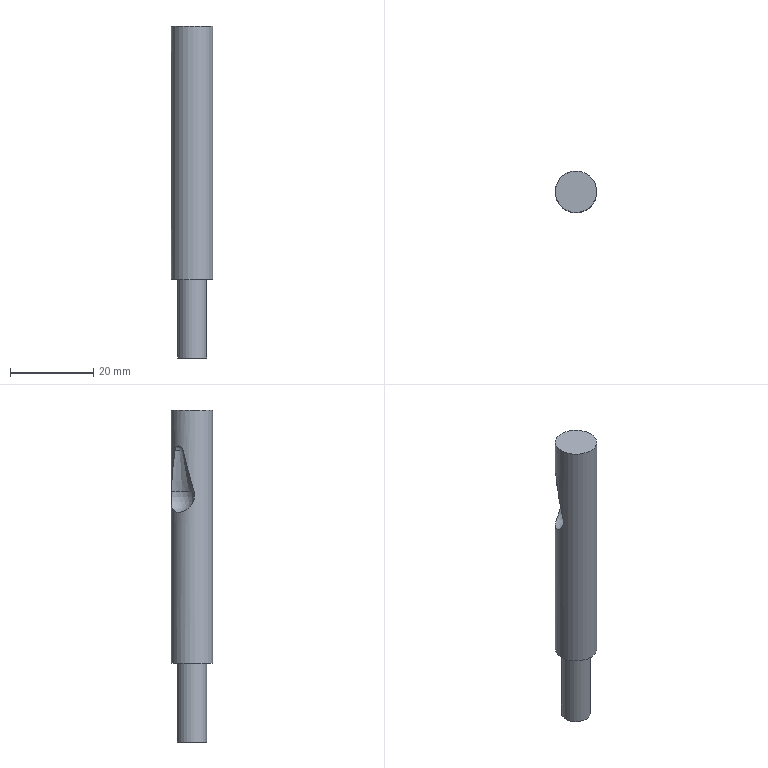Part | NX | features solid 2 | 1 solid | 8 faces | volume 5344 mm3 | plane 3 | cylinder 2 | sphere 2 | cone 1 | commonest cylinder face diameters 7 x1 10 x1